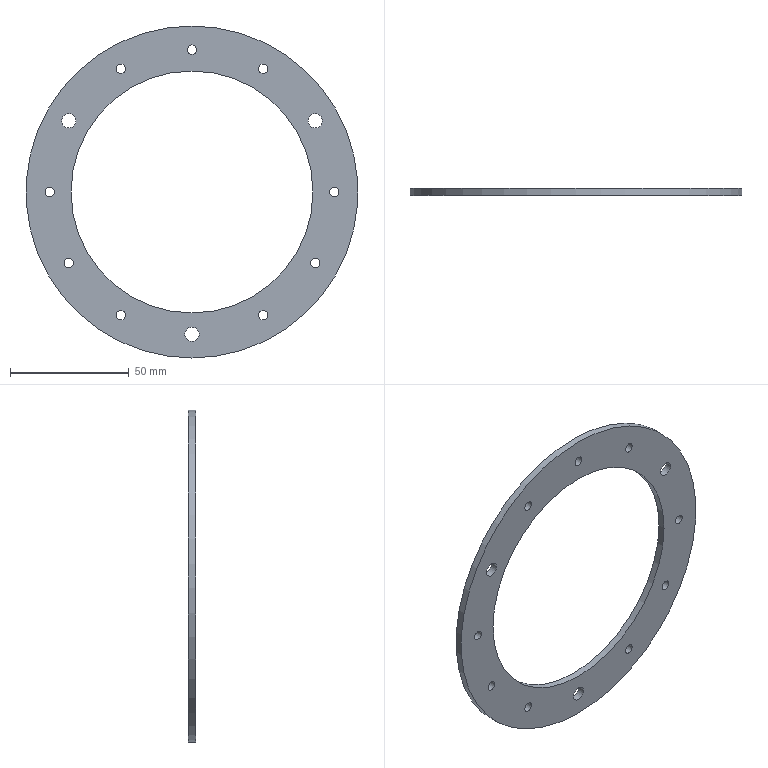Part | STEP file | JBJ-P-1018-03 | 1 solid | 16 faces | box 140 x 3 x 140 mm | volume 21074 mm3 | cylinder 14 | plane 2 | commonest cylinder face diameters 4 x9 6 x3 102 x1 140 x1
STEP:
#1=CARTESIAN_POINT('',(0.,3.,62.));
#2=VERTEX_POINT('',#1);
#3=CARTESIAN_POINT('',(0.,3.,60.));
#4=DIRECTION('',(0.,1.,0.));
#5=DIRECTION('',(0.,0.,1.));
#6=AXIS2_PLACEMENT_3D('',#3,#4,#5);
#7=CIRCLE('',#6,2.);
#8=EDGE_CURVE('',#2,#2,#7,.T.);
#9=ORIENTED_EDGE('',*,*,#8,.F.);
#10=EDGE_LOOP('',(#9));
#11=FACE_BOUND('',#10,.T.);
#12=CARTESIAN_POINT('',(60.,3.,2.));
#13=VERTEX_POINT('',#12);
#14=CARTESIAN_POINT('',(60.,3.,0.));
#15=DIRECTION('',(0.,1.,0.));
#16=DIRECTION('',(0.,0.,1.));
#17=AXIS2_PLACEMENT_3D('',#14,#15,#16);
#18=CIRCLE('',#17,2.);
#19=EDGE_CURVE('',#13,#13,#18,.T.);
#20=ORIENTED_EDGE('',*,*,#19,.F.);
#21=EDGE_LOOP('',(#20));
#22=FACE_BOUND('',#21,.T.);
#23=CARTESIAN_POINT('',(30.,3.,-49.962));
#24=VERTEX_POINT('',#23);
#25=CARTESIAN_POINT('',(30.,3.,-51.962));
#26=DIRECTION('',(0.,1.,0.));
#27=DIRECTION('',(0.,0.,1.));
#28=AXIS2_PLACEMENT_3D('',#25,#26,#27);
#29=CIRCLE('',#28,2.);
#30=EDGE_CURVE('',#24,#24,#29,.T.);
#31=ORIENTED_EDGE('',*,*,#30,.F.);
#32=EDGE_LOOP('',(#31));
#33=FACE_BOUND('',#32,.T.);
#34=CARTESIAN_POINT('',(-51.962,3.,-28.));
#35=VERTEX_POINT('',#34);
#36=CARTESIAN_POINT('',(-51.962,3.,-30.));
#37=DIRECTION('',(0.,1.,0.));
#38=DIRECTION('',(0.,0.,1.));
#39=AXIS2_PLACEMENT_3D('',#36,#37,#38);
#40=CIRCLE('',#39,2.);
#41=EDGE_CURVE('',#35,#35,#40,.T.);
#42=ORIENTED_EDGE('',*,*,#41,.F.);
#43=EDGE_LOOP('',(#42));
#44=FACE_BOUND('',#43,.T.);
#45=CARTESIAN_POINT('',(51.962,3.,33.));
#46=VERTEX_POINT('',#45);
#47=CARTESIAN_POINT('',(51.962,3.,30.));
#48=DIRECTION('',(0.,1.,0.));
#49=DIRECTION('',(0.,0.,1.));
#50=AXIS2_PLACEMENT_3D('',#47,#48,#49);
#51=CIRCLE('',#50,3.);
#52=EDGE_CURVE('',#46,#46,#51,.T.);
#53=ORIENTED_EDGE('',*,*,#52,.F.);
#54=EDGE_LOOP('',(#53));
#55=FACE_BOUND('',#54,.T.);
#56=CARTESIAN_POINT('',(0.,3.,-57.));
#57=VERTEX_POINT('',#56);
#58=CARTESIAN_POINT('',(0.,3.,-60.));
#59=DIRECTION('',(0.,1.,0.));
#60=DIRECTION('',(0.,0.,1.));
#61=AXIS2_PLACEMENT_3D('',#58,#59,#60);
#62=CIRCLE('',#61,3.);
#63=EDGE_CURVE('',#57,#57,#62,.T.);
#64=ORIENTED_EDGE('',*,*,#63,.F.);
#65=EDGE_LOOP('',(#64));
#66=FACE_BOUND('',#65,.T.);
#67=CARTESIAN_POINT('',(0.,3.,70.));
#68=VERTEX_POINT('',#67);
#69=CARTESIAN_POINT('',(0.,3.,0.));
#70=DIRECTION('',(0.,1.,0.));
#71=DIRECTION('',(0.,0.,1.));
#72=AXIS2_PLACEMENT_3D('',#69,#70,#71);
#73=CIRCLE('',#72,70.);
#74=EDGE_CURVE('',#68,#68,#73,.T.);
#75=ORIENTED_EDGE('',*,*,#74,.T.);
#76=EDGE_LOOP('',(#75));
#77=FACE_OUTER_BOUND('',#76,.T.);
#78=CARTESIAN_POINT('',(0.,3.,51.));
#79=VERTEX_POINT('',#78);
#80=CARTESIAN_POINT('',(0.,3.,0.));
#81=DIRECTION('',(0.,1.,0.));
#82=DIRECTION('',(0.,0.,1.));
#83=AXIS2_PLACEMENT_3D('',#80,#81,#82);
#84=CIRCLE('',#83,51.);
#85=EDGE_CURVE('',#79,#79,#84,.T.);
#86=ORIENTED_EDGE('',*,*,#85,.F.);
#87=EDGE_LOOP('',(#86));
#88=FACE_BOUND('',#87,.T.);
#89=CARTESIAN_POINT('',(-60.,3.,2.));
#90=VERTEX_POINT('',#89);
#91=CARTESIAN_POINT('',(-60.,3.,0.));
#92=DIRECTION('',(0.,1.,0.));
#93=DIRECTION('',(0.,0.,1.));
#94=AXIS2_PLACEMENT_3D('',#91,#92,#93);
#95=CIRCLE('',#94,2.);
#96=EDGE_CURVE('',#90,#90,#95,.T.);
#97=ORIENTED_EDGE('',*,*,#96,.F.);
#98=EDGE_LOOP('',(#97));
#99=FACE_BOUND('',#98,.T.);
#100=CARTESIAN_POINT('',(-51.962,3.,33.));
#101=VERTEX_POINT('',#100);
#102=CARTESIAN_POINT('',(-51.962,3.,30.));
#103=DIRECTION('',(0.,1.,0.));
#104=DIRECTION('',(0.,0.,1.));
#105=AXIS2_PLACEMENT_3D('',#102,#103,#104);
#106=CIRCLE('',#105,3.);
#107=EDGE_CURVE('',#101,#101,#106,.T.);
#108=ORIENTED_EDGE('',*,*,#107,.F.);
#109=EDGE_LOOP('',(#108));
#110=FACE_BOUND('',#109,.T.);
#111=CARTESIAN_POINT('',(-30.,3.,-49.962));
#112=VERTEX_POINT('',#111);
#113=CARTESIAN_POINT('',(-30.,3.,-51.962));
#114=DIRECTION('',(0.,1.,0.));
#115=DIRECTION('',(0.,0.,1.));
#116=AXIS2_PLACEMENT_3D('',#113,#114,#115);
#117=CIRCLE('',#116,2.);
#118=EDGE_CURVE('',#112,#112,#117,.T.);
#119=ORIENTED_EDGE('',*,*,#118,.F.);
#120=EDGE_LOOP('',(#119));
#121=FACE_BOUND('',#120,.T.);
#122=CARTESIAN_POINT('',(51.962,3.,-28.));
#123=VERTEX_POINT('',#122);
#124=CARTESIAN_POINT('',(51.962,3.,-30.));
#125=DIRECTION('',(0.,1.,0.));
#126=DIRECTION('',(0.,0.,1.));
#127=AXIS2_PLACEMENT_3D('',#124,#125,#126);
#128=CIRCLE('',#127,2.);
#129=EDGE_CURVE('',#123,#123,#128,.T.);
#130=ORIENTED_EDGE('',*,*,#129,.F.);
#131=EDGE_LOOP('',(#130));
#132=FACE_BOUND('',#131,.T.);
#133=CARTESIAN_POINT('',(30.,3.,53.962));
#134=VERTEX_POINT('',#133);
#135=CARTESIAN_POINT('',(30.,3.,51.962));
#136=DIRECTION('',(0.,1.,0.));
#137=DIRECTION('',(0.,0.,1.));
#138=AXIS2_PLACEMENT_3D('',#135,#136,#137);
#139=CIRCLE('',#138,2.);
#140=EDGE_CURVE('',#134,#134,#139,.T.);
#141=ORIENTED_EDGE('',*,*,#140,.F.);
#142=EDGE_LOOP('',(#141));
#143=FACE_BOUND('',#142,.T.);
#144=CARTESIAN_POINT('',(-30.,3.,53.962));
#145=VERTEX_POINT('',#144);
#146=CARTESIAN_POINT('',(-30.,3.,51.962));
#147=DIRECTION('',(0.,1.,0.));
#148=DIRECTION('',(0.,0.,1.));
#149=AXIS2_PLACEMENT_3D('',#146,#147,#148);
#150=CIRCLE('',#149,2.);
#151=EDGE_CURVE('',#145,#145,#150,.T.);
#152=ORIENTED_EDGE('',*,*,#151,.F.);
#153=EDGE_LOOP('',(#152));
#154=FACE_BOUND('',#153,.T.);
#155=CARTESIAN_POINT('',(0.,3.,0.));
#156=DIRECTION('',(0.,1.,0.));
#157=DIRECTION('',(0.,0.,1.));
#158=AXIS2_PLACEMENT_3D('',#155,#156,#157);
#159=PLANE('',#158);
#160=ADVANCED_FACE('',(#11,#22,#33,#44,#55,#66,#77,#88,#99,#110,#121,#132,#143,#154),#159,.T.);
#161=CARTESIAN_POINT('',(0.,0.,70.));
#162=VERTEX_POINT('',#161);
#163=CARTESIAN_POINT('',(0.,0.,0.));
#164=DIRECTION('',(0.,1.,0.));
#165=DIRECTION('',(0.,0.,1.));
#166=AXIS2_PLACEMENT_3D('',#163,#164,#165);
#167=CIRCLE('',#166,70.);
#168=EDGE_CURVE('',#162,#162,#167,.T.);
#169=ORIENTED_EDGE('',*,*,#168,.F.);
#170=EDGE_LOOP('',(#169));
#171=FACE_OUTER_BOUND('',#170,.T.);
#172=CARTESIAN_POINT('',(0.,0.,51.));
#173=VERTEX_POINT('',#172);
#174=CARTESIAN_POINT('',(0.,0.,0.));
#175=DIRECTION('',(0.,1.,0.));
#176=DIRECTION('',(0.,0.,1.));
#177=AXIS2_PLACEMENT_3D('',#174,#175,#176);
#178=CIRCLE('',#177,51.);
#179=EDGE_CURVE('',#173,#173,#178,.T.);
#180=ORIENTED_EDGE('',*,*,#179,.T.);
#181=EDGE_LOOP('',(#180));
#182=FACE_BOUND('',#181,.T.);
#183=CARTESIAN_POINT('',(0.,0.,-57.));
#184=VERTEX_POINT('',#183);
#185=CARTESIAN_POINT('',(0.,0.,-60.));
#186=DIRECTION('',(0.,1.,0.));
#187=DIRECTION('',(0.,0.,1.));
#188=AXIS2_PLACEMENT_3D('',#185,#186,#187);
#189=CIRCLE('',#188,3.);
#190=EDGE_CURVE('',#184,#184,#189,.T.);
#191=ORIENTED_EDGE('',*,*,#190,.T.);
#192=EDGE_LOOP('',(#191));
#193=FACE_BOUND('',#192,.T.);
#194=CARTESIAN_POINT('',(-60.,0.,2.));
#195=VERTEX_POINT('',#194);
#196=CARTESIAN_POINT('',(-60.,0.,0.));
#197=DIRECTION('',(0.,1.,0.));
#198=DIRECTION('',(0.,0.,1.));
#199=AXIS2_PLACEMENT_3D('',#196,#197,#198);
#200=CIRCLE('',#199,2.);
#201=EDGE_CURVE('',#195,#195,#200,.T.);
#202=ORIENTED_EDGE('',*,*,#201,.T.);
#203=EDGE_LOOP('',(#202));
#204=FACE_BOUND('',#203,.T.);
#205=CARTESIAN_POINT('',(51.962,0.,33.));
#206=VERTEX_POINT('',#205);
#207=CARTESIAN_POINT('',(51.962,0.,30.));
#208=DIRECTION('',(0.,1.,0.));
#209=DIRECTION('',(0.,0.,1.));
#210=AXIS2_PLACEMENT_3D('',#207,#208,#209);
#211=CIRCLE('',#210,3.);
#212=EDGE_CURVE('',#206,#206,#211,.T.);
#213=ORIENTED_EDGE('',*,*,#212,.T.);
#214=EDGE_LOOP('',(#213));
#215=FACE_BOUND('',#214,.T.);
#216=CARTESIAN_POINT('',(-51.962,0.,33.));
#217=VERTEX_POINT('',#216);
#218=CARTESIAN_POINT('',(-51.962,0.,30.));
#219=DIRECTION('',(0.,1.,0.));
#220=DIRECTION('',(0.,0.,1.));
#221=AXIS2_PLACEMENT_3D('',#218,#219,#220);
#222=CIRCLE('',#221,3.);
#223=EDGE_CURVE('',#217,#217,#222,.T.);
#224=ORIENTED_EDGE('',*,*,#223,.T.);
#225=EDGE_LOOP('',(#224));
#226=FACE_BOUND('',#225,.T.);
#227=CARTESIAN_POINT('',(-51.962,0.,-28.));
#228=VERTEX_POINT('',#227);
#229=CARTESIAN_POINT('',(-51.962,0.,-30.));
#230=DIRECTION('',(0.,1.,0.));
#231=DIRECTION('',(0.,0.,1.));
#232=AXIS2_PLACEMENT_3D('',#229,#230,#231);
#233=CIRCLE('',#232,2.);
#234=EDGE_CURVE('',#228,#228,#233,.T.);
#235=ORIENTED_EDGE('',*,*,#234,.T.);
#236=EDGE_LOOP('',(#235));
#237=FACE_BOUND('',#236,.T.);
#238=CARTESIAN_POINT('',(-30.,0.,-49.962));
#239=VERTEX_POINT('',#238);
#240=CARTESIAN_POINT('',(-30.,0.,-51.962));
#241=DIRECTION('',(0.,1.,0.));
#242=DIRECTION('',(0.,0.,1.));
#243=AXIS2_PLACEMENT_3D('',#240,#241,#242);
#244=CIRCLE('',#243,2.);
#245=EDGE_CURVE('',#239,#239,#244,.T.);
#246=ORIENTED_EDGE('',*,*,#245,.T.);
#247=EDGE_LOOP('',(#246));
#248=FACE_BOUND('',#247,.T.);
#249=CARTESIAN_POINT('',(30.,0.,-49.962));
#250=VERTEX_POINT('',#249);
#251=CARTESIAN_POINT('',(30.,0.,-51.962));
#252=DIRECTION('',(0.,1.,0.));
#253=DIRECTION('',(0.,0.,1.));
#254=AXIS2_PLACEMENT_3D('',#251,#252,#253);
#255=CIRCLE('',#254,2.);
#256=EDGE_CURVE('',#250,#250,#255,.T.);
#257=ORIENTED_EDGE('',*,*,#256,.T.);
#258=EDGE_LOOP('',(#257));
#259=FACE_BOUND('',#258,.T.);
#260=CARTESIAN_POINT('',(51.962,0.,-28.));
#261=VERTEX_POINT('',#260);
#262=CARTESIAN_POINT('',(51.962,0.,-30.));
#263=DIRECTION('',(0.,1.,0.));
#264=DIRECTION('',(0.,0.,1.));
#265=AXIS2_PLACEMENT_3D('',#262,#263,#264);
#266=CIRCLE('',#265,2.);
#267=EDGE_CURVE('',#261,#261,#266,.T.);
#268=ORIENTED_EDGE('',*,*,#267,.T.);
#269=EDGE_LOOP('',(#268));
#270=FACE_BOUND('',#269,.T.);
#271=CARTESIAN_POINT('',(60.,0.,2.));
#272=VERTEX_POINT('',#271);
#273=CARTESIAN_POINT('',(60.,0.,0.));
#274=DIRECTION('',(0.,1.,0.));
#275=DIRECTION('',(0.,0.,1.));
#276=AXIS2_PLACEMENT_3D('',#273,#274,#275);
#277=CIRCLE('',#276,2.);
#278=EDGE_CURVE('',#272,#272,#277,.T.);
#279=ORIENTED_EDGE('',*,*,#278,.T.);
#280=EDGE_LOOP('',(#279));
#281=FACE_BOUND('',#280,.T.);
#282=CARTESIAN_POINT('',(30.,0.,53.962));
#283=VERTEX_POINT('',#282);
#284=CARTESIAN_POINT('',(30.,0.,51.962));
#285=DIRECTION('',(0.,1.,0.));
#286=DIRECTION('',(0.,0.,1.));
#287=AXIS2_PLACEMENT_3D('',#284,#285,#286);
#288=CIRCLE('',#287,2.);
#289=EDGE_CURVE('',#283,#283,#288,.T.);
#290=ORIENTED_EDGE('',*,*,#289,.T.);
#291=EDGE_LOOP('',(#290));
#292=FACE_BOUND('',#291,.T.);
#293=CARTESIAN_POINT('',(0.,0.,62.));
#294=VERTEX_POINT('',#293);
#295=CARTESIAN_POINT('',(0.,0.,60.));
#296=DIRECTION('',(0.,1.,0.));
#297=DIRECTION('',(0.,0.,1.));
#298=AXIS2_PLACEMENT_3D('',#295,#296,#297);
#299=CIRCLE('',#298,2.);
#300=EDGE_CURVE('',#294,#294,#299,.T.);
#301=ORIENTED_EDGE('',*,*,#300,.T.);
#302=EDGE_LOOP('',(#301));
#303=FACE_BOUND('',#302,.T.);
#304=CARTESIAN_POINT('',(-30.,0.,53.962));
#305=VERTEX_POINT('',#304);
#306=CARTESIAN_POINT('',(-30.,0.,51.962));
#307=DIRECTION('',(0.,1.,0.));
#308=DIRECTION('',(0.,0.,1.));
#309=AXIS2_PLACEMENT_3D('',#306,#307,#308);
#310=CIRCLE('',#309,2.);
#311=EDGE_CURVE('',#305,#305,#310,.T.);
#312=ORIENTED_EDGE('',*,*,#311,.T.);
#313=EDGE_LOOP('',(#312));
#314=FACE_BOUND('',#313,.T.);
#315=CARTESIAN_POINT('',(0.,0.,0.));
#316=DIRECTION('',(0.,1.,0.));
#317=DIRECTION('',(0.,0.,1.));
#318=AXIS2_PLACEMENT_3D('',#315,#316,#317);
#319=PLANE('',#318);
#320=ADVANCED_FACE('',(#171,#182,#193,#204,#215,#226,#237,#248,#259,#270,#281,#292,#303,#314),#319,.F.);
#321=ORIENTED_EDGE('',*,*,#74,.F.);
#322=EDGE_LOOP('',(#321));
#323=FACE_OUTER_BOUND('',#322,.T.);
#324=ORIENTED_EDGE('',*,*,#168,.T.);
#325=EDGE_LOOP('',(#324));
#326=FACE_OUTER_BOUND('',#325,.T.);
#327=CARTESIAN_POINT('',(0.,3.,0.));
#328=DIRECTION('',(0.,-1.,0.));
#329=DIRECTION('',(0.,0.,-1.));
#330=AXIS2_PLACEMENT_3D('',#327,#328,#329);
#331=CYLINDRICAL_SURFACE('',#330,70.);
#332=ADVANCED_FACE('',(#323,#326),#331,.T.);
#333=ORIENTED_EDGE('',*,*,#85,.T.);
#334=EDGE_LOOP('',(#333));
#335=FACE_OUTER_BOUND('',#334,.T.);
#336=ORIENTED_EDGE('',*,*,#179,.F.);
#337=EDGE_LOOP('',(#336));
#338=FACE_OUTER_BOUND('',#337,.T.);
#339=CARTESIAN_POINT('',(0.,3.,0.));
#340=DIRECTION('',(0.,-1.,0.));
#341=DIRECTION('',(0.,0.,-1.));
#342=AXIS2_PLACEMENT_3D('',#339,#340,#341);
#343=CYLINDRICAL_SURFACE('',#342,51.);
#344=ADVANCED_FACE('',(#335,#338),#343,.F.);
#345=ORIENTED_EDGE('',*,*,#63,.T.);
#346=EDGE_LOOP('',(#345));
#347=FACE_OUTER_BOUND('',#346,.T.);
#348=ORIENTED_EDGE('',*,*,#190,.F.);
#349=EDGE_LOOP('',(#348));
#350=FACE_OUTER_BOUND('',#349,.T.);
#351=CARTESIAN_POINT('',(0.,3.,-60.));
#352=DIRECTION('',(0.,-1.,0.));
#353=DIRECTION('',(0.,0.,-1.));
#354=AXIS2_PLACEMENT_3D('',#351,#352,#353);
#355=CYLINDRICAL_SURFACE('',#354,3.);
#356=ADVANCED_FACE('',(#347,#350),#355,.F.);
#357=ORIENTED_EDGE('',*,*,#96,.T.);
#358=EDGE_LOOP('',(#357));
#359=FACE_OUTER_BOUND('',#358,.T.);
#360=ORIENTED_EDGE('',*,*,#201,.F.);
#361=EDGE_LOOP('',(#360));
#362=FACE_OUTER_BOUND('',#361,.T.);
#363=CARTESIAN_POINT('',(-60.,3.,0.));
#364=DIRECTION('',(0.,-1.,0.));
#365=DIRECTION('',(0.,0.,-1.));
#366=AXIS2_PLACEMENT_3D('',#363,#364,#365);
#367=CYLINDRICAL_SURFACE('',#366,2.);
#368=ADVANCED_FACE('',(#359,#362),#367,.F.);
#369=ORIENTED_EDGE('',*,*,#52,.T.);
#370=EDGE_LOOP('',(#369));
#371=FACE_OUTER_BOUND('',#370,.T.);
#372=ORIENTED_EDGE('',*,*,#212,.F.);
#373=EDGE_LOOP('',(#372));
#374=FACE_OUTER_BOUND('',#373,.T.);
#375=CARTESIAN_POINT('',(51.962,3.,30.));
#376=DIRECTION('',(0.,-1.,0.));
#377=DIRECTION('',(0.,0.,-1.));
#378=AXIS2_PLACEMENT_3D('',#375,#376,#377);
#379=CYLINDRICAL_SURFACE('',#378,3.);
#380=ADVANCED_FACE('',(#371,#374),#379,.F.);
#381=ORIENTED_EDGE('',*,*,#107,.T.);
#382=EDGE_LOOP('',(#381));
#383=FACE_OUTER_BOUND('',#382,.T.);
#384=ORIENTED_EDGE('',*,*,#223,.F.);
#385=EDGE_LOOP('',(#384));
#386=FACE_OUTER_BOUND('',#385,.T.);
#387=CARTESIAN_POINT('',(-51.962,3.,30.));
#388=DIRECTION('',(0.,-1.,0.));
#389=DIRECTION('',(0.,0.,-1.));
#390=AXIS2_PLACEMENT_3D('',#387,#388,#389);
#391=CYLINDRICAL_SURFACE('',#390,3.);
#392=ADVANCED_FACE('',(#383,#386),#391,.F.);
#393=ORIENTED_EDGE('',*,*,#41,.T.);
#394=EDGE_LOOP('',(#393));
#395=FACE_OUTER_BOUND('',#394,.T.);
#396=ORIENTED_EDGE('',*,*,#234,.F.);
#397=EDGE_LOOP('',(#396));
#398=FACE_OUTER_BOUND('',#397,.T.);
#399=CARTESIAN_POINT('',(-51.962,3.,-30.));
#400=DIRECTION('',(0.,-1.,0.));
#401=DIRECTION('',(0.,0.,-1.));
#402=AXIS2_PLACEMENT_3D('',#399,#400,#401);
#403=CYLINDRICAL_SURFACE('',#402,2.);
#404=ADVANCED_FACE('',(#395,#398),#403,.F.);
#405=ORIENTED_EDGE('',*,*,#118,.T.);
#406=EDGE_LOOP('',(#405));
#407=FACE_OUTER_BOUND('',#406,.T.);
#408=ORIENTED_EDGE('',*,*,#245,.F.);
#409=EDGE_LOOP('',(#408));
#410=FACE_OUTER_BOUND('',#409,.T.);
#411=CARTESIAN_POINT('',(-30.,3.,-51.962));
#412=DIRECTION('',(0.,-1.,0.));
#413=DIRECTION('',(0.,0.,-1.));
#414=AXIS2_PLACEMENT_3D('',#411,#412,#413);
#415=CYLINDRICAL_SURFACE('',#414,2.);
#416=ADVANCED_FACE('',(#407,#410),#415,.F.);
#417=ORIENTED_EDGE('',*,*,#30,.T.);
#418=EDGE_LOOP('',(#417));
#419=FACE_OUTER_BOUND('',#418,.T.);
#420=ORIENTED_EDGE('',*,*,#256,.F.);
#421=EDGE_LOOP('',(#420));
#422=FACE_OUTER_BOUND('',#421,.T.);
#423=CARTESIAN_POINT('',(30.,3.,-51.962));
#424=DIRECTION('',(0.,-1.,0.));
#425=DIRECTION('',(0.,0.,-1.));
#426=AXIS2_PLACEMENT_3D('',#423,#424,#425);
#427=CYLINDRICAL_SURFACE('',#426,2.);
#428=ADVANCED_FACE('',(#419,#422),#427,.F.);
#429=ORIENTED_EDGE('',*,*,#129,.T.);
#430=EDGE_LOOP('',(#429));
#431=FACE_OUTER_BOUND('',#430,.T.);
#432=ORIENTED_EDGE('',*,*,#267,.F.);
#433=EDGE_LOOP('',(#432));
#434=FACE_OUTER_BOUND('',#433,.T.);
#435=CARTESIAN_POINT('',(51.962,3.,-30.));
#436=DIRECTION('',(0.,-1.,0.));
#437=DIRECTION('',(0.,0.,-1.));
#438=AXIS2_PLACEMENT_3D('',#435,#436,#437);
#439=CYLINDRICAL_SURFACE('',#438,2.);
#440=ADVANCED_FACE('',(#431,#434),#439,.F.);
#441=ORIENTED_EDGE('',*,*,#19,.T.);
#442=EDGE_LOOP('',(#441));
#443=FACE_OUTER_BOUND('',#442,.T.);
#444=ORIENTED_EDGE('',*,*,#278,.F.);
#445=EDGE_LOOP('',(#444));
#446=FACE_OUTER_BOUND('',#445,.T.);
#447=CARTESIAN_POINT('',(60.,3.,0.));
#448=DIRECTION('',(0.,-1.,0.));
#449=DIRECTION('',(0.,0.,-1.));
#450=AXIS2_PLACEMENT_3D('',#447,#448,#449);
#451=CYLINDRICAL_SURFACE('',#450,2.);
#452=ADVANCED_FACE('',(#443,#446),#451,.F.);
#453=ORIENTED_EDGE('',*,*,#140,.T.);
#454=EDGE_LOOP('',(#453));
#455=FACE_OUTER_BOUND('',#454,.T.);
#456=ORIENTED_EDGE('',*,*,#289,.F.);
#457=EDGE_LOOP('',(#456));
#458=FACE_OUTER_BOUND('',#457,.T.);
#459=CARTESIAN_POINT('',(30.,3.,51.962));
#460=DIRECTION('',(0.,-1.,0.));
#461=DIRECTION('',(0.,0.,-1.));
#462=AXIS2_PLACEMENT_3D('',#459,#460,#461);
#463=CYLINDRICAL_SURFACE('',#462,2.);
#464=ADVANCED_FACE('',(#455,#458),#463,.F.);
#465=ORIENTED_EDGE('',*,*,#8,.T.);
#466=EDGE_LOOP('',(#465));
#467=FACE_OUTER_BOUND('',#466,.T.);
#468=ORIENTED_EDGE('',*,*,#300,.F.);
#469=EDGE_LOOP('',(#468));
#470=FACE_OUTER_BOUND('',#469,.T.);
#471=CARTESIAN_POINT('',(0.,3.,60.));
#472=DIRECTION('',(0.,-1.,0.));
#473=DIRECTION('',(0.,0.,-1.));
#474=AXIS2_PLACEMENT_3D('',#471,#472,#473);
#475=CYLINDRICAL_SURFACE('',#474,2.);
#476=ADVANCED_FACE('',(#467,#470),#475,.F.);
#477=ORIENTED_EDGE('',*,*,#151,.T.);
#478=EDGE_LOOP('',(#477));
#479=FACE_OUTER_BOUND('',#478,.T.);
#480=ORIENTED_EDGE('',*,*,#311,.F.);
#481=EDGE_LOOP('',(#480));
#482=FACE_OUTER_BOUND('',#481,.T.);
#483=CARTESIAN_POINT('',(-30.,3.,51.962));
#484=DIRECTION('',(0.,-1.,0.));
#485=DIRECTION('',(0.,0.,-1.));
#486=AXIS2_PLACEMENT_3D('',#483,#484,#485);
#487=CYLINDRICAL_SURFACE('',#486,2.);
#488=ADVANCED_FACE('',(#479,#482),#487,.F.);
#489=CLOSED_SHELL('',(#160,#320,#332,#344,#356,#368,#380,#392,#404,#416,#428,#440,#452,#464,#476,#488));
#490=MANIFOLD_SOLID_BREP('',#489);
#491=CARTESIAN_POINT('',(0.,0.,0.));
#492=DIRECTION('',(0.,0.,1.));
#493=DIRECTION('',(1.,0.,0.));
#494=AXIS2_PLACEMENT_3D('',#491,#492,#493);
#495=(LENGTH_UNIT()NAMED_UNIT(*)SI_UNIT(.MILLI.,.METRE.));
#496=UNCERTAINTY_MEASURE_WITH_UNIT(LENGTH_MEASURE(0.00001),#495,'','');
#497=(NAMED_UNIT(*)PLANE_ANGLE_UNIT()SI_UNIT($,.RADIAN.));
#498=(NAMED_UNIT(*)SI_UNIT($,.STERADIAN.)SOLID_ANGLE_UNIT());
#499=(GEOMETRIC_REPRESENTATION_CONTEXT(3)GLOBAL_UNCERTAINTY_ASSIGNED_CONTEXT((#496))GLOBAL_UNIT_ASSIGNED_CONTEXT((#495,#497,#498))REPRESENTATION_CONTEXT('',''));
#500=ADVANCED_BREP_SHAPE_REPRESENTATION('',(#490,#494),#499);